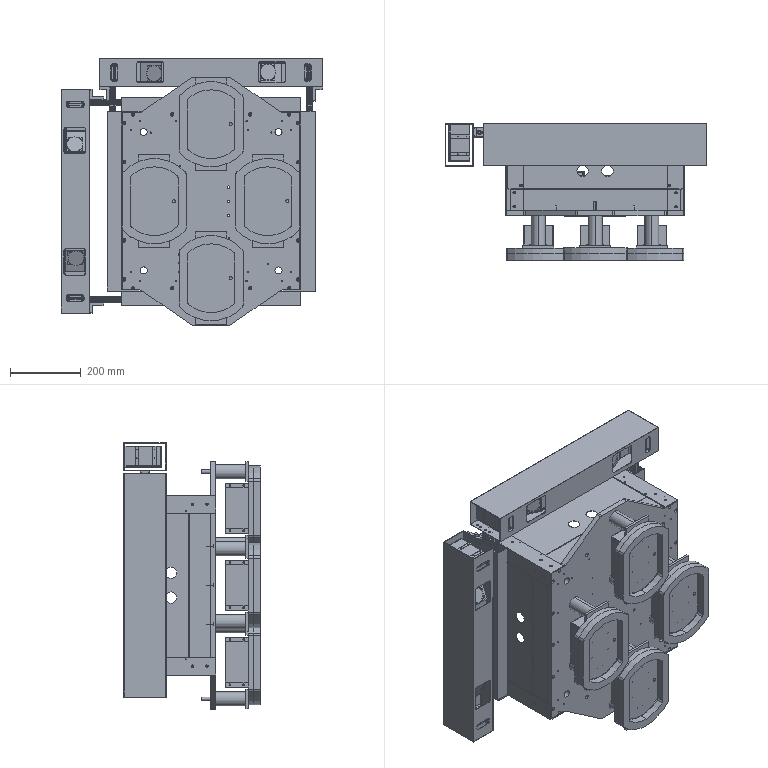Part | SolidWorks | features CompositeCurve 32, InContextFeatHolder 24 | 159 solids | 15107 faces | volume 22718189 mm3 | plane 8291 | cylinder 4806 | cone 1075 | spline 828 | sphere 58 | torus 49 | commonest cylinder face diameters 1 x603 5.5 x392 2 x362 4.2 x344 0.2 x292 3.3 x188